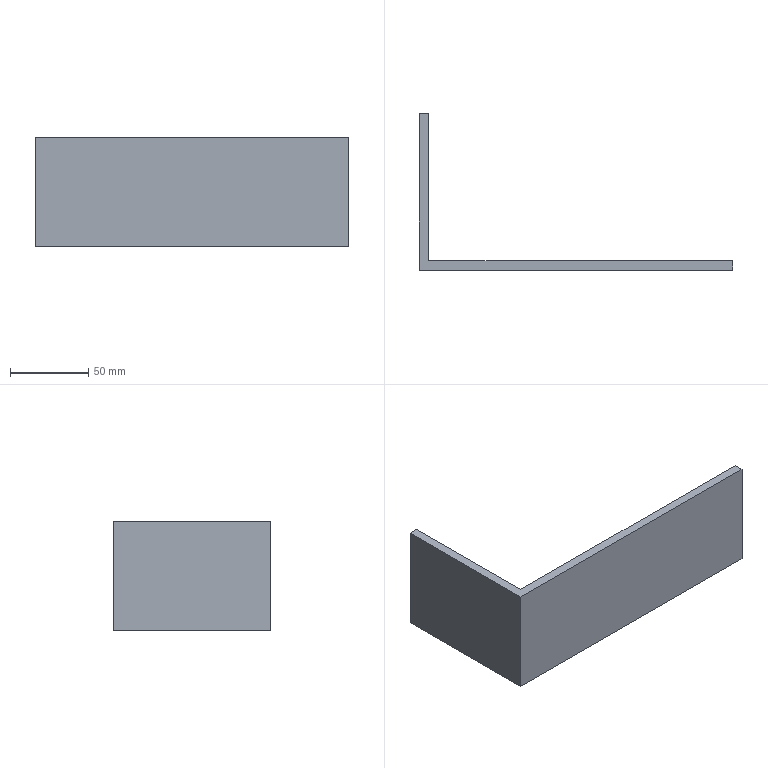Part | SolidWorks | features Extrusion 1 | 1 solid | 8 faces | box 200 x 100 x 70 mm | volume 123480 mm3 | plane 8
STEP:
#1=CARTESIAN_POINT('',(6.,0.,0.));
#2=VERTEX_POINT('',#1);
#3=CARTESIAN_POINT('',(0.,0.,0.));
#4=VERTEX_POINT('',#3);
#5=CARTESIAN_POINT('',(0.,0.,0.));
#6=DIRECTION('',(-1.,0.,0.));
#7=VECTOR('',#6,1000.);
#8=LINE('',#5,#7);
#9=EDGE_CURVE('',#2,#4,#8,.T.);
#10=ORIENTED_EDGE('',*,*,#9,.T.);
#11=CARTESIAN_POINT('',(0.,0.,70.));
#12=VERTEX_POINT('',#11);
#13=CARTESIAN_POINT('',(0.,0.,70.));
#14=DIRECTION('',(0.,0.,-1.));
#15=VECTOR('',#14,1000.);
#16=LINE('',#13,#15);
#17=EDGE_CURVE('',#12,#4,#16,.T.);
#18=ORIENTED_EDGE('',*,*,#17,.F.);
#19=CARTESIAN_POINT('',(6.,0.,70.));
#20=VERTEX_POINT('',#19);
#21=CARTESIAN_POINT('',(0.,0.,70.));
#22=DIRECTION('',(-1.,0.,0.));
#23=VECTOR('',#22,1000.);
#24=LINE('',#21,#23);
#25=EDGE_CURVE('',#20,#12,#24,.T.);
#26=ORIENTED_EDGE('',*,*,#25,.F.);
#27=CARTESIAN_POINT('',(6.,0.,70.));
#28=DIRECTION('',(0.,0.,-1.));
#29=VECTOR('',#28,1000.);
#30=LINE('',#27,#29);
#31=EDGE_CURVE('',#20,#2,#30,.T.);
#32=ORIENTED_EDGE('',*,*,#31,.T.);
#33=EDGE_LOOP('',(#10,#18,#26,#32));
#34=FACE_OUTER_BOUND('',#33,.T.);
#35=CARTESIAN_POINT('',(0.,0.,70.));
#36=DIRECTION('',(0.,-1.,0.));
#37=DIRECTION('',(0.,0.,-1.));
#38=AXIS2_PLACEMENT_3D('',#35,#36,#37);
#39=PLANE('',#38);
#40=ADVANCED_FACE('',(#34),#39,.F.);
#41=CARTESIAN_POINT('',(0.,-100.,0.));
#42=VERTEX_POINT('',#41);
#43=CARTESIAN_POINT('',(0.,0.,0.));
#44=DIRECTION('',(0.,-1.,0.));
#45=VECTOR('',#44,1000.);
#46=LINE('',#43,#45);
#47=EDGE_CURVE('',#4,#42,#46,.T.);
#48=ORIENTED_EDGE('',*,*,#47,.T.);
#49=CARTESIAN_POINT('',(0.,-100.,70.));
#50=VERTEX_POINT('',#49);
#51=CARTESIAN_POINT('',(0.,-100.,70.));
#52=DIRECTION('',(0.,0.,-1.));
#53=VECTOR('',#52,1000.);
#54=LINE('',#51,#53);
#55=EDGE_CURVE('',#50,#42,#54,.T.);
#56=ORIENTED_EDGE('',*,*,#55,.F.);
#57=CARTESIAN_POINT('',(0.,0.,70.));
#58=DIRECTION('',(0.,-1.,0.));
#59=VECTOR('',#58,1000.);
#60=LINE('',#57,#59);
#61=EDGE_CURVE('',#12,#50,#60,.T.);
#62=ORIENTED_EDGE('',*,*,#61,.F.);
#63=ORIENTED_EDGE('',*,*,#17,.T.);
#64=EDGE_LOOP('',(#48,#56,#62,#63));
#65=FACE_OUTER_BOUND('',#64,.T.);
#66=CARTESIAN_POINT('',(0.,0.,70.));
#67=DIRECTION('',(1.,0.,0.));
#68=DIRECTION('',(0.,1.,0.));
#69=AXIS2_PLACEMENT_3D('',#66,#67,#68);
#70=PLANE('',#69);
#71=ADVANCED_FACE('',(#65),#70,.F.);
#72=CARTESIAN_POINT('',(200.,-100.,0.));
#73=VERTEX_POINT('',#72);
#74=CARTESIAN_POINT('',(0.,-100.,0.));
#75=DIRECTION('',(1.,0.,0.));
#76=VECTOR('',#75,1000.);
#77=LINE('',#74,#76);
#78=EDGE_CURVE('',#42,#73,#77,.T.);
#79=ORIENTED_EDGE('',*,*,#78,.T.);
#80=CARTESIAN_POINT('',(200.,-100.,70.));
#81=VERTEX_POINT('',#80);
#82=CARTESIAN_POINT('',(200.,-100.,70.));
#83=DIRECTION('',(0.,0.,-1.));
#84=VECTOR('',#83,1000.);
#85=LINE('',#82,#84);
#86=EDGE_CURVE('',#81,#73,#85,.T.);
#87=ORIENTED_EDGE('',*,*,#86,.F.);
#88=CARTESIAN_POINT('',(0.,-100.,70.));
#89=DIRECTION('',(1.,0.,0.));
#90=VECTOR('',#89,1000.);
#91=LINE('',#88,#90);
#92=EDGE_CURVE('',#50,#81,#91,.T.);
#93=ORIENTED_EDGE('',*,*,#92,.F.);
#94=ORIENTED_EDGE('',*,*,#55,.T.);
#95=EDGE_LOOP('',(#79,#87,#93,#94));
#96=FACE_OUTER_BOUND('',#95,.T.);
#97=CARTESIAN_POINT('',(0.,-100.,70.));
#98=DIRECTION('',(0.,1.,0.));
#99=DIRECTION('',(0.,0.,1.));
#100=AXIS2_PLACEMENT_3D('',#97,#98,#99);
#101=PLANE('',#100);
#102=ADVANCED_FACE('',(#96),#101,.F.);
#103=CARTESIAN_POINT('',(200.,-94.,0.));
#104=VERTEX_POINT('',#103);
#105=CARTESIAN_POINT('',(200.,-100.,0.));
#106=DIRECTION('',(0.,1.,0.));
#107=VECTOR('',#106,1000.);
#108=LINE('',#105,#107);
#109=EDGE_CURVE('',#73,#104,#108,.T.);
#110=ORIENTED_EDGE('',*,*,#109,.T.);
#111=CARTESIAN_POINT('',(200.,-94.,70.));
#112=VERTEX_POINT('',#111);
#113=CARTESIAN_POINT('',(200.,-94.,70.));
#114=DIRECTION('',(0.,0.,-1.));
#115=VECTOR('',#114,1000.);
#116=LINE('',#113,#115);
#117=EDGE_CURVE('',#112,#104,#116,.T.);
#118=ORIENTED_EDGE('',*,*,#117,.F.);
#119=CARTESIAN_POINT('',(200.,-100.,70.));
#120=DIRECTION('',(0.,1.,0.));
#121=VECTOR('',#120,1000.);
#122=LINE('',#119,#121);
#123=EDGE_CURVE('',#81,#112,#122,.T.);
#124=ORIENTED_EDGE('',*,*,#123,.F.);
#125=ORIENTED_EDGE('',*,*,#86,.T.);
#126=EDGE_LOOP('',(#110,#118,#124,#125));
#127=FACE_OUTER_BOUND('',#126,.T.);
#128=CARTESIAN_POINT('',(200.,-100.,70.));
#129=DIRECTION('',(-1.,0.,0.));
#130=DIRECTION('',(0.,0.,1.));
#131=AXIS2_PLACEMENT_3D('',#128,#129,#130);
#132=PLANE('',#131);
#133=ADVANCED_FACE('',(#127),#132,.F.);
#134=CARTESIAN_POINT('',(6.,-94.,0.));
#135=VERTEX_POINT('',#134);
#136=CARTESIAN_POINT('',(6.,-94.,0.));
#137=DIRECTION('',(-1.,0.,0.));
#138=VECTOR('',#137,1000.);
#139=LINE('',#136,#138);
#140=EDGE_CURVE('',#104,#135,#139,.T.);
#141=ORIENTED_EDGE('',*,*,#140,.T.);
#142=CARTESIAN_POINT('',(6.,-94.,70.));
#143=VERTEX_POINT('',#142);
#144=CARTESIAN_POINT('',(6.,-94.,70.));
#145=DIRECTION('',(0.,0.,-1.));
#146=VECTOR('',#145,1000.);
#147=LINE('',#144,#146);
#148=EDGE_CURVE('',#143,#135,#147,.T.);
#149=ORIENTED_EDGE('',*,*,#148,.F.);
#150=CARTESIAN_POINT('',(6.,-94.,70.));
#151=DIRECTION('',(-1.,0.,0.));
#152=VECTOR('',#151,1000.);
#153=LINE('',#150,#152);
#154=EDGE_CURVE('',#112,#143,#153,.T.);
#155=ORIENTED_EDGE('',*,*,#154,.F.);
#156=ORIENTED_EDGE('',*,*,#117,.T.);
#157=EDGE_LOOP('',(#141,#149,#155,#156));
#158=FACE_OUTER_BOUND('',#157,.T.);
#159=CARTESIAN_POINT('',(6.,-94.,70.));
#160=DIRECTION('',(0.,-1.,0.));
#161=DIRECTION('',(0.,0.,-1.));
#162=AXIS2_PLACEMENT_3D('',#159,#160,#161);
#163=PLANE('',#162);
#164=ADVANCED_FACE('',(#158),#163,.F.);
#165=CARTESIAN_POINT('',(6.,0.,0.));
#166=DIRECTION('',(0.,1.,0.));
#167=VECTOR('',#166,1000.);
#168=LINE('',#165,#167);
#169=EDGE_CURVE('',#135,#2,#168,.T.);
#170=ORIENTED_EDGE('',*,*,#169,.T.);
#171=ORIENTED_EDGE('',*,*,#31,.F.);
#172=CARTESIAN_POINT('',(6.,0.,70.));
#173=DIRECTION('',(0.,1.,0.));
#174=VECTOR('',#173,1000.);
#175=LINE('',#172,#174);
#176=EDGE_CURVE('',#143,#20,#175,.T.);
#177=ORIENTED_EDGE('',*,*,#176,.F.);
#178=ORIENTED_EDGE('',*,*,#148,.T.);
#179=EDGE_LOOP('',(#170,#171,#177,#178));
#180=FACE_OUTER_BOUND('',#179,.T.);
#181=CARTESIAN_POINT('',(6.,0.,70.));
#182=DIRECTION('',(-1.,0.,0.));
#183=DIRECTION('',(0.,0.,1.));
#184=AXIS2_PLACEMENT_3D('',#181,#182,#183);
#185=PLANE('',#184);
#186=ADVANCED_FACE('',(#180),#185,.F.);
#187=ORIENTED_EDGE('',*,*,#25,.T.);
#188=ORIENTED_EDGE('',*,*,#61,.T.);
#189=ORIENTED_EDGE('',*,*,#92,.T.);
#190=ORIENTED_EDGE('',*,*,#123,.T.);
#191=ORIENTED_EDGE('',*,*,#154,.T.);
#192=ORIENTED_EDGE('',*,*,#176,.T.);
#193=EDGE_LOOP('',(#187,#188,#189,#190,#191,#192));
#194=FACE_OUTER_BOUND('',#193,.T.);
#195=CARTESIAN_POINT('',(0.,0.,70.));
#196=DIRECTION('',(0.,0.,-1.));
#197=DIRECTION('',(-1.,0.,0.));
#198=AXIS2_PLACEMENT_3D('',#195,#196,#197);
#199=PLANE('',#198);
#200=ADVANCED_FACE('',(#194),#199,.F.);
#201=ORIENTED_EDGE('',*,*,#9,.F.);
#202=ORIENTED_EDGE('',*,*,#169,.F.);
#203=ORIENTED_EDGE('',*,*,#140,.F.);
#204=ORIENTED_EDGE('',*,*,#109,.F.);
#205=ORIENTED_EDGE('',*,*,#78,.F.);
#206=ORIENTED_EDGE('',*,*,#47,.F.);
#207=EDGE_LOOP('',(#201,#202,#203,#204,#205,#206));
#208=FACE_OUTER_BOUND('',#207,.T.);
#209=CARTESIAN_POINT('',(0.,0.,0.));
#210=DIRECTION('',(0.,0.,-1.));
#211=DIRECTION('',(-1.,0.,0.));
#212=AXIS2_PLACEMENT_3D('',#209,#210,#211);
#213=PLANE('',#212);
#214=ADVANCED_FACE('',(#208),#213,.T.);
#215=CLOSED_SHELL('',(#40,#71,#102,#133,#164,#186,#200,#214));
#216=MANIFOLD_SOLID_BREP('',#215);
#217=CARTESIAN_POINT('',(0.,0.,0.));
#218=DIRECTION('',(0.,0.,1.));
#219=DIRECTION('',(1.,0.,0.));
#220=AXIS2_PLACEMENT_3D('',#217,#218,#219);
#221=(LENGTH_UNIT()NAMED_UNIT(*)SI_UNIT(.MILLI.,.METRE.));
#222=UNCERTAINTY_MEASURE_WITH_UNIT(LENGTH_MEASURE(0.00001),#221,'','');
#223=(NAMED_UNIT(*)PLANE_ANGLE_UNIT()SI_UNIT($,.RADIAN.));
#224=(NAMED_UNIT(*)SI_UNIT($,.STERADIAN.)SOLID_ANGLE_UNIT());
#225=(GEOMETRIC_REPRESENTATION_CONTEXT(3)GLOBAL_UNCERTAINTY_ASSIGNED_CONTEXT((#222))GLOBAL_UNIT_ASSIGNED_CONTEXT((#221,#223,#224))REPRESENTATION_CONTEXT('',''));
#226=ADVANCED_BREP_SHAPE_REPRESENTATION('',(#216,#220),#225);